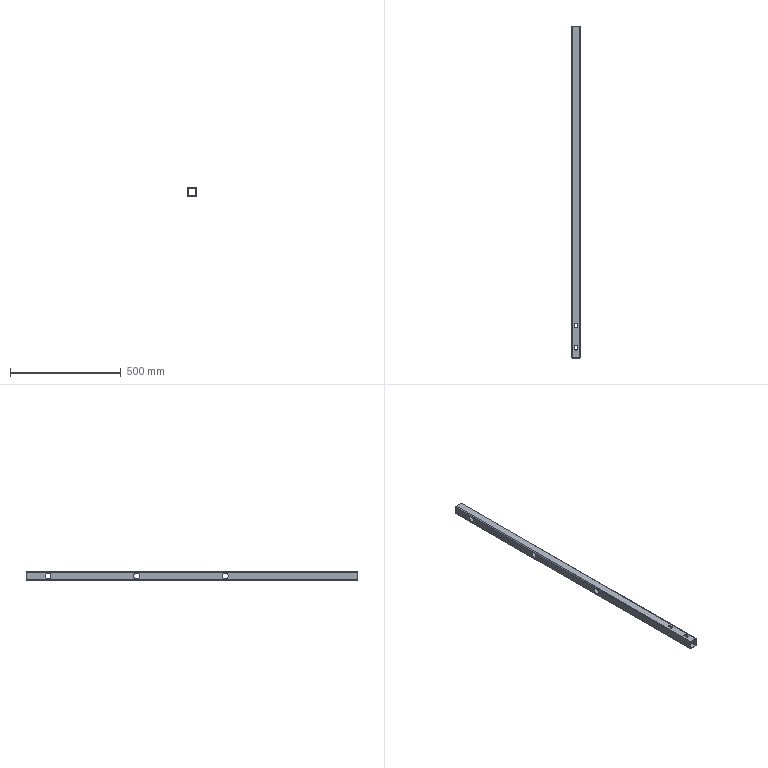Part | STEP file | 护栏立柱2主体_Default<As Machined> | 1 solid | 46 faces | box 40 x 1500 x 40 mm | volume 432313 mm3 | cylinder 28 | plane 18 | commonest cylinder face diameters 26 x12 12 x8 4 x4 8 x4